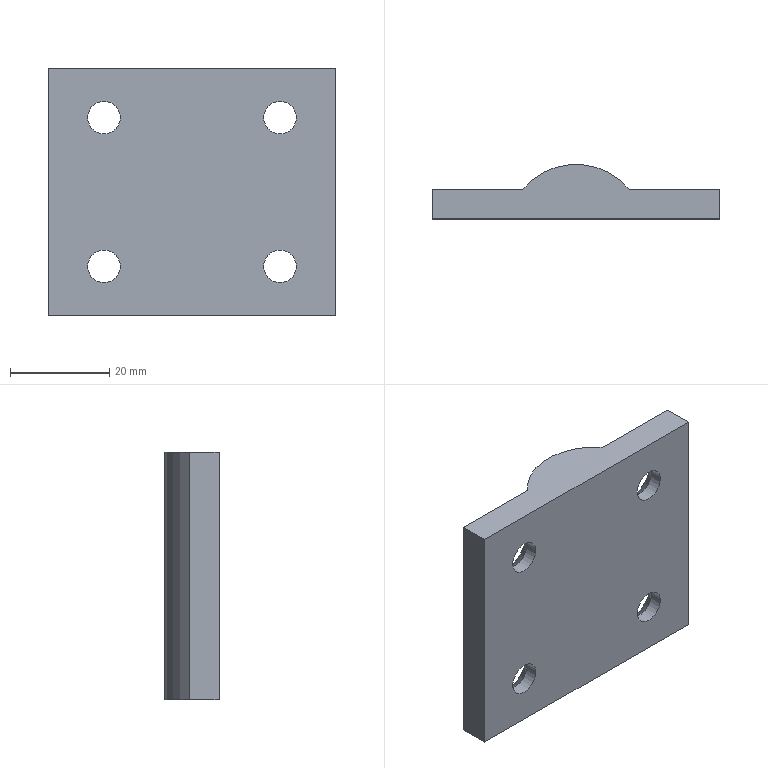Part | SolidWorks | features BaseBody 1 | 1 solid | 24 faces | box 58 x 11 x 50 mm | volume 19652 mm3 | cylinder 9 | cone 8 | plane 7 | commonest cylinder face diameters 6.6 x8 28 x1
STEP:
#1=CARTESIAN_POINT('',(43.45,0.,10.));
#2=VERTEX_POINT('',#1);
#3=CARTESIAN_POINT('',(50.05,0.,10.));
#4=VERTEX_POINT('',#3);
#5=CARTESIAN_POINT('',(46.75,0.,10.));
#6=DIRECTION('',(0.,-1.,0.));
#7=DIRECTION('',(-1.,0.,0.));
#8=AXIS2_PLACEMENT_3D('',#5,#6,#7);
#9=CIRCLE('',#8,3.3);
#10=EDGE_CURVE('',#2,#4,#9,.T.);
#11=ORIENTED_EDGE('',*,*,#10,.T.);
#12=CARTESIAN_POINT('',(50.05,2.58,10.));
#13=VERTEX_POINT('',#12);
#14=CARTESIAN_POINT('',(50.05,6.,10.));
#15=DIRECTION('',(0.,1.,0.));
#16=VECTOR('',#15,1000.);
#17=LINE('',#14,#16);
#18=EDGE_CURVE('',#4,#13,#17,.T.);
#19=ORIENTED_EDGE('',*,*,#18,.T.);
#20=CARTESIAN_POINT('',(43.45,2.58,10.));
#21=VERTEX_POINT('',#20);
#22=CARTESIAN_POINT('',(46.75,2.58,10.));
#23=DIRECTION('',(0.,-1.,0.));
#24=DIRECTION('',(-1.,0.,0.));
#25=AXIS2_PLACEMENT_3D('',#22,#23,#24);
#26=CIRCLE('',#25,3.3);
#27=EDGE_CURVE('',#21,#13,#26,.T.);
#28=ORIENTED_EDGE('',*,*,#27,.F.);
#29=CARTESIAN_POINT('',(43.45,6.,10.));
#30=DIRECTION('',(0.,1.,0.));
#31=VECTOR('',#30,1000.);
#32=LINE('',#29,#31);
#33=EDGE_CURVE('',#2,#21,#32,.T.);
#34=ORIENTED_EDGE('',*,*,#33,.F.);
#35=EDGE_LOOP('',(#11,#19,#28,#34));
#36=FACE_OUTER_BOUND('',#35,.T.);
#37=CARTESIAN_POINT('',(46.75,6.,10.));
#38=DIRECTION('',(0.,1.,0.));
#39=DIRECTION('',(-1.,0.,0.));
#40=AXIS2_PLACEMENT_3D('',#37,#38,#39);
#41=CYLINDRICAL_SURFACE('',#40,3.3);
#42=ADVANCED_FACE('',(#36),#41,.F.);
#43=CARTESIAN_POINT('',(43.45,0.,40.));
#44=VERTEX_POINT('',#43);
#45=CARTESIAN_POINT('',(50.05,0.,40.));
#46=VERTEX_POINT('',#45);
#47=CARTESIAN_POINT('',(46.75,0.,40.));
#48=DIRECTION('',(0.,-1.,0.));
#49=DIRECTION('',(-1.,0.,0.));
#50=AXIS2_PLACEMENT_3D('',#47,#48,#49);
#51=CIRCLE('',#50,3.3);
#52=EDGE_CURVE('',#44,#46,#51,.T.);
#53=ORIENTED_EDGE('',*,*,#52,.T.);
#54=CARTESIAN_POINT('',(50.05,2.58,40.));
#55=VERTEX_POINT('',#54);
#56=CARTESIAN_POINT('',(50.05,6.,40.));
#57=DIRECTION('',(0.,1.,0.));
#58=VECTOR('',#57,1000.);
#59=LINE('',#56,#58);
#60=EDGE_CURVE('',#46,#55,#59,.T.);
#61=ORIENTED_EDGE('',*,*,#60,.T.);
#62=CARTESIAN_POINT('',(43.45,2.58,40.));
#63=VERTEX_POINT('',#62);
#64=CARTESIAN_POINT('',(46.75,2.58,40.));
#65=DIRECTION('',(0.,-1.,0.));
#66=DIRECTION('',(-1.,0.,0.));
#67=AXIS2_PLACEMENT_3D('',#64,#65,#66);
#68=CIRCLE('',#67,3.3);
#69=EDGE_CURVE('',#63,#55,#68,.T.);
#70=ORIENTED_EDGE('',*,*,#69,.F.);
#71=CARTESIAN_POINT('',(43.45,6.,40.));
#72=DIRECTION('',(0.,1.,0.));
#73=VECTOR('',#72,1000.);
#74=LINE('',#71,#73);
#75=EDGE_CURVE('',#44,#63,#74,.T.);
#76=ORIENTED_EDGE('',*,*,#75,.F.);
#77=EDGE_LOOP('',(#53,#61,#70,#76));
#78=FACE_OUTER_BOUND('',#77,.T.);
#79=CARTESIAN_POINT('',(46.75,6.,40.));
#80=DIRECTION('',(0.,1.,0.));
#81=DIRECTION('',(-1.,0.,0.));
#82=AXIS2_PLACEMENT_3D('',#79,#80,#81);
#83=CYLINDRICAL_SURFACE('',#82,3.3);
#84=ADVANCED_FACE('',(#78),#83,.F.);
#85=CARTESIAN_POINT('',(7.95,0.,40.));
#86=VERTEX_POINT('',#85);
#87=CARTESIAN_POINT('',(14.55,0.,40.));
#88=VERTEX_POINT('',#87);
#89=CARTESIAN_POINT('',(11.25,0.,40.));
#90=DIRECTION('',(0.,-1.,0.));
#91=DIRECTION('',(-1.,0.,0.));
#92=AXIS2_PLACEMENT_3D('',#89,#90,#91);
#93=CIRCLE('',#92,3.3);
#94=EDGE_CURVE('',#86,#88,#93,.T.);
#95=ORIENTED_EDGE('',*,*,#94,.T.);
#96=CARTESIAN_POINT('',(14.55,2.58,40.));
#97=VERTEX_POINT('',#96);
#98=CARTESIAN_POINT('',(14.55,6.,40.));
#99=DIRECTION('',(0.,1.,0.));
#100=VECTOR('',#99,1000.);
#101=LINE('',#98,#100);
#102=EDGE_CURVE('',#88,#97,#101,.T.);
#103=ORIENTED_EDGE('',*,*,#102,.T.);
#104=CARTESIAN_POINT('',(7.95,2.58,40.));
#105=VERTEX_POINT('',#104);
#106=CARTESIAN_POINT('',(11.25,2.58,40.));
#107=DIRECTION('',(0.,-1.,0.));
#108=DIRECTION('',(-1.,0.,0.));
#109=AXIS2_PLACEMENT_3D('',#106,#107,#108);
#110=CIRCLE('',#109,3.3);
#111=EDGE_CURVE('',#105,#97,#110,.T.);
#112=ORIENTED_EDGE('',*,*,#111,.F.);
#113=CARTESIAN_POINT('',(7.95,6.,40.));
#114=DIRECTION('',(0.,1.,0.));
#115=VECTOR('',#114,1000.);
#116=LINE('',#113,#115);
#117=EDGE_CURVE('',#86,#105,#116,.T.);
#118=ORIENTED_EDGE('',*,*,#117,.F.);
#119=EDGE_LOOP('',(#95,#103,#112,#118));
#120=FACE_OUTER_BOUND('',#119,.T.);
#121=CARTESIAN_POINT('',(11.25,6.,40.));
#122=DIRECTION('',(0.,1.,0.));
#123=DIRECTION('',(-1.,0.,0.));
#124=AXIS2_PLACEMENT_3D('',#121,#122,#123);
#125=CYLINDRICAL_SURFACE('',#124,3.3);
#126=ADVANCED_FACE('',(#120),#125,.F.);
#127=CARTESIAN_POINT('',(7.95,0.,10.));
#128=VERTEX_POINT('',#127);
#129=CARTESIAN_POINT('',(14.55,0.,10.));
#130=VERTEX_POINT('',#129);
#131=CARTESIAN_POINT('',(11.25,0.,10.));
#132=DIRECTION('',(0.,-1.,0.));
#133=DIRECTION('',(-1.,0.,0.));
#134=AXIS2_PLACEMENT_3D('',#131,#132,#133);
#135=CIRCLE('',#134,3.3);
#136=EDGE_CURVE('',#128,#130,#135,.T.);
#137=ORIENTED_EDGE('',*,*,#136,.T.);
#138=CARTESIAN_POINT('',(14.55,2.58,10.));
#139=VERTEX_POINT('',#138);
#140=CARTESIAN_POINT('',(14.55,6.,10.));
#141=DIRECTION('',(0.,1.,0.));
#142=VECTOR('',#141,1000.);
#143=LINE('',#140,#142);
#144=EDGE_CURVE('',#130,#139,#143,.T.);
#145=ORIENTED_EDGE('',*,*,#144,.T.);
#146=CARTESIAN_POINT('',(7.95,2.58,10.));
#147=VERTEX_POINT('',#146);
#148=CARTESIAN_POINT('',(11.25,2.58,10.));
#149=DIRECTION('',(0.,-1.,0.));
#150=DIRECTION('',(-1.,0.,0.));
#151=AXIS2_PLACEMENT_3D('',#148,#149,#150);
#152=CIRCLE('',#151,3.3);
#153=EDGE_CURVE('',#147,#139,#152,.T.);
#154=ORIENTED_EDGE('',*,*,#153,.F.);
#155=CARTESIAN_POINT('',(7.95,6.,10.));
#156=DIRECTION('',(0.,1.,0.));
#157=VECTOR('',#156,1000.);
#158=LINE('',#155,#157);
#159=EDGE_CURVE('',#128,#147,#158,.T.);
#160=ORIENTED_EDGE('',*,*,#159,.F.);
#161=EDGE_LOOP('',(#137,#145,#154,#160));
#162=FACE_OUTER_BOUND('',#161,.T.);
#163=CARTESIAN_POINT('',(11.25,6.,10.));
#164=DIRECTION('',(0.,1.,0.));
#165=DIRECTION('',(-1.,0.,0.));
#166=AXIS2_PLACEMENT_3D('',#163,#164,#165);
#167=CYLINDRICAL_SURFACE('',#166,3.3);
#168=ADVANCED_FACE('',(#162),#167,.F.);
#169=ORIENTED_EDGE('',*,*,#27,.T.);
#170=CARTESIAN_POINT('',(53.47,6.,10.));
#171=VERTEX_POINT('',#170);
#172=CARTESIAN_POINT('',(53.47,6.,10.));
#173=DIRECTION('',(0.7071,0.7071,0.));
#174=VECTOR('',#173,1000.);
#175=LINE('',#172,#174);
#176=EDGE_CURVE('',#13,#171,#175,.T.);
#177=ORIENTED_EDGE('',*,*,#176,.T.);
#178=CARTESIAN_POINT('',(40.03,6.,10.));
#179=VERTEX_POINT('',#178);
#180=CARTESIAN_POINT('',(46.75,6.,10.));
#181=DIRECTION('',(0.,1.,0.));
#182=DIRECTION('',(-1.,0.,0.));
#183=AXIS2_PLACEMENT_3D('',#180,#181,#182);
#184=CIRCLE('',#183,6.72);
#185=EDGE_CURVE('',#171,#179,#184,.T.);
#186=ORIENTED_EDGE('',*,*,#185,.T.);
#187=CARTESIAN_POINT('',(40.03,6.,10.));
#188=DIRECTION('',(-0.7071,0.7071,0.));
#189=VECTOR('',#188,1000.);
#190=LINE('',#187,#189);
#191=EDGE_CURVE('',#21,#179,#190,.T.);
#192=ORIENTED_EDGE('',*,*,#191,.F.);
#193=EDGE_LOOP('',(#169,#177,#186,#192));
#194=FACE_OUTER_BOUND('',#193,.T.);
#195=CARTESIAN_POINT('',(46.75,6.,10.));
#196=DIRECTION('',(0.,1.,0.));
#197=DIRECTION('',(-1.,0.,0.));
#198=AXIS2_PLACEMENT_3D('',#195,#196,#197);
#199=CONICAL_SURFACE('',#198,6.72,0.7854);
#200=ADVANCED_FACE('',(#194),#199,.F.);
#201=ORIENTED_EDGE('',*,*,#69,.T.);
#202=CARTESIAN_POINT('',(53.47,6.,40.));
#203=VERTEX_POINT('',#202);
#204=CARTESIAN_POINT('',(53.47,6.,40.));
#205=DIRECTION('',(0.7071,0.7071,0.));
#206=VECTOR('',#205,1000.);
#207=LINE('',#204,#206);
#208=EDGE_CURVE('',#55,#203,#207,.T.);
#209=ORIENTED_EDGE('',*,*,#208,.T.);
#210=CARTESIAN_POINT('',(40.03,6.,40.));
#211=VERTEX_POINT('',#210);
#212=CARTESIAN_POINT('',(46.75,6.,40.));
#213=DIRECTION('',(0.,1.,0.));
#214=DIRECTION('',(-1.,0.,0.));
#215=AXIS2_PLACEMENT_3D('',#212,#213,#214);
#216=CIRCLE('',#215,6.72);
#217=EDGE_CURVE('',#203,#211,#216,.T.);
#218=ORIENTED_EDGE('',*,*,#217,.T.);
#219=CARTESIAN_POINT('',(40.03,6.,40.));
#220=DIRECTION('',(-0.7071,0.7071,0.));
#221=VECTOR('',#220,1000.);
#222=LINE('',#219,#221);
#223=EDGE_CURVE('',#63,#211,#222,.T.);
#224=ORIENTED_EDGE('',*,*,#223,.F.);
#225=EDGE_LOOP('',(#201,#209,#218,#224));
#226=FACE_OUTER_BOUND('',#225,.T.);
#227=CARTESIAN_POINT('',(46.75,6.,40.));
#228=DIRECTION('',(0.,1.,0.));
#229=DIRECTION('',(-1.,0.,0.));
#230=AXIS2_PLACEMENT_3D('',#227,#228,#229);
#231=CONICAL_SURFACE('',#230,6.72,0.7854);
#232=ADVANCED_FACE('',(#226),#231,.F.);
#233=ORIENTED_EDGE('',*,*,#111,.T.);
#234=CARTESIAN_POINT('',(17.97,6.,40.));
#235=VERTEX_POINT('',#234);
#236=CARTESIAN_POINT('',(17.97,6.,40.));
#237=DIRECTION('',(0.7071,0.7071,0.));
#238=VECTOR('',#237,1000.);
#239=LINE('',#236,#238);
#240=EDGE_CURVE('',#97,#235,#239,.T.);
#241=ORIENTED_EDGE('',*,*,#240,.T.);
#242=CARTESIAN_POINT('',(4.53,6.,40.));
#243=VERTEX_POINT('',#242);
#244=CARTESIAN_POINT('',(11.25,6.,40.));
#245=DIRECTION('',(0.,1.,0.));
#246=DIRECTION('',(-1.,0.,0.));
#247=AXIS2_PLACEMENT_3D('',#244,#245,#246);
#248=CIRCLE('',#247,6.72);
#249=EDGE_CURVE('',#235,#243,#248,.T.);
#250=ORIENTED_EDGE('',*,*,#249,.T.);
#251=CARTESIAN_POINT('',(4.53,6.,40.));
#252=DIRECTION('',(-0.7071,0.7071,0.));
#253=VECTOR('',#252,1000.);
#254=LINE('',#251,#253);
#255=EDGE_CURVE('',#105,#243,#254,.T.);
#256=ORIENTED_EDGE('',*,*,#255,.F.);
#257=EDGE_LOOP('',(#233,#241,#250,#256));
#258=FACE_OUTER_BOUND('',#257,.T.);
#259=CARTESIAN_POINT('',(11.25,6.,40.));
#260=DIRECTION('',(0.,1.,0.));
#261=DIRECTION('',(-1.,0.,0.));
#262=AXIS2_PLACEMENT_3D('',#259,#260,#261);
#263=CONICAL_SURFACE('',#262,6.72,0.7854);
#264=ADVANCED_FACE('',(#258),#263,.F.);
#265=ORIENTED_EDGE('',*,*,#153,.T.);
#266=CARTESIAN_POINT('',(17.97,6.,10.));
#267=VERTEX_POINT('',#266);
#268=CARTESIAN_POINT('',(17.97,6.,10.));
#269=DIRECTION('',(0.7071,0.7071,0.));
#270=VECTOR('',#269,1000.);
#271=LINE('',#268,#270);
#272=EDGE_CURVE('',#139,#267,#271,.T.);
#273=ORIENTED_EDGE('',*,*,#272,.T.);
#274=CARTESIAN_POINT('',(4.53,6.,10.));
#275=VERTEX_POINT('',#274);
#276=CARTESIAN_POINT('',(11.25,6.,10.));
#277=DIRECTION('',(0.,1.,0.));
#278=DIRECTION('',(-1.,0.,0.));
#279=AXIS2_PLACEMENT_3D('',#276,#277,#278);
#280=CIRCLE('',#279,6.72);
#281=EDGE_CURVE('',#267,#275,#280,.T.);
#282=ORIENTED_EDGE('',*,*,#281,.T.);
#283=CARTESIAN_POINT('',(4.53,6.,10.));
#284=DIRECTION('',(-0.7071,0.7071,0.));
#285=VECTOR('',#284,1000.);
#286=LINE('',#283,#285);
#287=EDGE_CURVE('',#147,#275,#286,.T.);
#288=ORIENTED_EDGE('',*,*,#287,.F.);
#289=EDGE_LOOP('',(#265,#273,#282,#288));
#290=FACE_OUTER_BOUND('',#289,.T.);
#291=CARTESIAN_POINT('',(11.25,6.,10.));
#292=DIRECTION('',(0.,1.,0.));
#293=DIRECTION('',(-1.,0.,0.));
#294=AXIS2_PLACEMENT_3D('',#291,#292,#293);
#295=CONICAL_SURFACE('',#294,6.72,0.7854);
#296=ADVANCED_FACE('',(#290),#295,.F.);
#297=CARTESIAN_POINT('',(58.,0.,50.));
#298=VERTEX_POINT('',#297);
#299=CARTESIAN_POINT('',(58.,0.,0.));
#300=VERTEX_POINT('',#299);
#301=CARTESIAN_POINT('',(58.,0.,50.));
#302=DIRECTION('',(0.,0.,-1.));
#303=VECTOR('',#302,1000.);
#304=LINE('',#301,#303);
#305=EDGE_CURVE('',#298,#300,#304,.T.);
#306=ORIENTED_EDGE('',*,*,#305,.F.);
#307=CARTESIAN_POINT('',(0.,0.,50.));
#308=VERTEX_POINT('',#307);
#309=CARTESIAN_POINT('',(0.,0.,50.));
#310=DIRECTION('',(1.,0.,0.));
#311=VECTOR('',#310,1000.);
#312=LINE('',#309,#311);
#313=EDGE_CURVE('',#308,#298,#312,.T.);
#314=ORIENTED_EDGE('',*,*,#313,.F.);
#315=CARTESIAN_POINT('',(0.,0.,0.));
#316=VERTEX_POINT('',#315);
#317=CARTESIAN_POINT('',(0.,0.,50.));
#318=DIRECTION('',(0.,0.,1.));
#319=VECTOR('',#318,1000.);
#320=LINE('',#317,#319);
#321=EDGE_CURVE('',#316,#308,#320,.T.);
#322=ORIENTED_EDGE('',*,*,#321,.F.);
#323=CARTESIAN_POINT('',(0.,0.,0.));
#324=DIRECTION('',(-1.,0.,0.));
#325=VECTOR('',#324,1000.);
#326=LINE('',#323,#325);
#327=EDGE_CURVE('',#300,#316,#326,.T.);
#328=ORIENTED_EDGE('',*,*,#327,.F.);
#329=EDGE_LOOP('',(#306,#314,#322,#328));
#330=FACE_OUTER_BOUND('',#329,.T.);
#331=ORIENTED_EDGE('',*,*,#10,.F.);
#332=CARTESIAN_POINT('',(46.75,0.,10.));
#333=DIRECTION('',(0.,-1.,0.));
#334=DIRECTION('',(-1.,0.,0.));
#335=AXIS2_PLACEMENT_3D('',#332,#333,#334);
#336=CIRCLE('',#335,3.3);
#337=EDGE_CURVE('',#4,#2,#336,.T.);
#338=ORIENTED_EDGE('',*,*,#337,.F.);
#339=EDGE_LOOP('',(#331,#338));
#340=FACE_BOUND('',#339,.T.);
#341=ORIENTED_EDGE('',*,*,#52,.F.);
#342=CARTESIAN_POINT('',(46.75,0.,40.));
#343=DIRECTION('',(0.,-1.,0.));
#344=DIRECTION('',(-1.,0.,0.));
#345=AXIS2_PLACEMENT_3D('',#342,#343,#344);
#346=CIRCLE('',#345,3.3);
#347=EDGE_CURVE('',#46,#44,#346,.T.);
#348=ORIENTED_EDGE('',*,*,#347,.F.);
#349=EDGE_LOOP('',(#341,#348));
#350=FACE_BOUND('',#349,.T.);
#351=ORIENTED_EDGE('',*,*,#94,.F.);
#352=CARTESIAN_POINT('',(11.25,0.,40.));
#353=DIRECTION('',(0.,-1.,0.));
#354=DIRECTION('',(-1.,0.,0.));
#355=AXIS2_PLACEMENT_3D('',#352,#353,#354);
#356=CIRCLE('',#355,3.3);
#357=EDGE_CURVE('',#88,#86,#356,.T.);
#358=ORIENTED_EDGE('',*,*,#357,.F.);
#359=EDGE_LOOP('',(#351,#358));
#360=FACE_BOUND('',#359,.T.);
#361=ORIENTED_EDGE('',*,*,#136,.F.);
#362=CARTESIAN_POINT('',(11.25,0.,10.));
#363=DIRECTION('',(0.,-1.,0.));
#364=DIRECTION('',(-1.,0.,0.));
#365=AXIS2_PLACEMENT_3D('',#362,#363,#364);
#366=CIRCLE('',#365,3.3);
#367=EDGE_CURVE('',#130,#128,#366,.T.);
#368=ORIENTED_EDGE('',*,*,#367,.F.);
#369=EDGE_LOOP('',(#361,#368));
#370=FACE_BOUND('',#369,.T.);
#371=CARTESIAN_POINT('',(0.,0.,50.));
#372=DIRECTION('',(0.,1.,0.));
#373=DIRECTION('',(-1.,0.,0.));
#374=AXIS2_PLACEMENT_3D('',#371,#372,#373);
#375=PLANE('',#374);
#376=ADVANCED_FACE('',(#330,#340,#350,#360,#370),#375,.F.);
#377=CARTESIAN_POINT('',(18.276,6.,0.));
#378=VERTEX_POINT('',#377);
#379=CARTESIAN_POINT('',(0.,6.,0.));
#380=VERTEX_POINT('',#379);
#381=CARTESIAN_POINT('',(29.,6.,0.));
#382=DIRECTION('',(-1.,0.,0.));
#383=VECTOR('',#382,1000.);
#384=LINE('',#381,#383);
#385=EDGE_CURVE('',#378,#380,#384,.T.);
#386=ORIENTED_EDGE('',*,*,#385,.F.);
#387=CARTESIAN_POINT('',(39.724,6.,0.));
#388=VERTEX_POINT('',#387);
#389=CARTESIAN_POINT('',(29.,-3.,0.));
#390=DIRECTION('',(0.,0.,1.));
#391=DIRECTION('',(-1.,0.,0.));
#392=AXIS2_PLACEMENT_3D('',#389,#390,#391);
#393=CIRCLE('',#392,14.);
#394=EDGE_CURVE('',#388,#378,#393,.T.);
#395=ORIENTED_EDGE('',*,*,#394,.F.);
#396=CARTESIAN_POINT('',(58.,6.,0.));
#397=VERTEX_POINT('',#396);
#398=CARTESIAN_POINT('',(29.,6.,0.));
#399=DIRECTION('',(-1.,0.,0.));
#400=VECTOR('',#399,1000.);
#401=LINE('',#398,#400);
#402=EDGE_CURVE('',#397,#388,#401,.T.);
#403=ORIENTED_EDGE('',*,*,#402,.F.);
#404=CARTESIAN_POINT('',(58.,-3.,0.));
#405=DIRECTION('',(0.,1.,0.));
#406=VECTOR('',#405,1000.);
#407=LINE('',#404,#406);
#408=EDGE_CURVE('',#300,#397,#407,.T.);
#409=ORIENTED_EDGE('',*,*,#408,.F.);
#410=ORIENTED_EDGE('',*,*,#327,.T.);
#411=CARTESIAN_POINT('',(0.,-3.,0.));
#412=DIRECTION('',(0.,-1.,0.));
#413=VECTOR('',#412,1000.);
#414=LINE('',#411,#413);
#415=EDGE_CURVE('',#380,#316,#414,.T.);
#416=ORIENTED_EDGE('',*,*,#415,.F.);
#417=EDGE_LOOP('',(#386,#395,#403,#409,#410,#416));
#418=FACE_OUTER_BOUND('',#417,.T.);
#419=CARTESIAN_POINT('',(29.,-3.,0.));
#420=DIRECTION('',(0.,0.,1.));
#421=DIRECTION('',(1.,0.,0.));
#422=AXIS2_PLACEMENT_3D('',#419,#420,#421);
#423=PLANE('',#422);
#424=ADVANCED_FACE('',(#418),#423,.F.);
#425=CARTESIAN_POINT('',(58.,6.,50.));
#426=VERTEX_POINT('',#425);
#427=CARTESIAN_POINT('',(58.,6.,50.));
#428=DIRECTION('',(0.,0.,-1.));
#429=VECTOR('',#428,1000.);
#430=LINE('',#427,#429);
#431=EDGE_CURVE('',#426,#397,#430,.T.);
#432=ORIENTED_EDGE('',*,*,#431,.F.);
#433=CARTESIAN_POINT('',(58.,0.,50.));
#434=DIRECTION('',(0.,1.,0.));
#435=VECTOR('',#434,1000.);
#436=LINE('',#433,#435);
#437=EDGE_CURVE('',#298,#426,#436,.T.);
#438=ORIENTED_EDGE('',*,*,#437,.F.);
#439=ORIENTED_EDGE('',*,*,#305,.T.);
#440=ORIENTED_EDGE('',*,*,#408,.T.);
#441=EDGE_LOOP('',(#432,#438,#439,#440));
#442=FACE_OUTER_BOUND('',#441,.T.);
#443=CARTESIAN_POINT('',(58.,0.,50.));
#444=DIRECTION('',(-1.,0.,0.));
#445=DIRECTION('',(0.,0.,1.));
#446=AXIS2_PLACEMENT_3D('',#443,#444,#445);
#447=PLANE('',#446);
#448=ADVANCED_FACE('',(#442),#447,.F.);
#449=CARTESIAN_POINT('',(39.724,6.,50.));
#450=VERTEX_POINT('',#449);
#451=CARTESIAN_POINT('',(18.276,6.,50.));
#452=VERTEX_POINT('',#451);
#453=CARTESIAN_POINT('',(29.,-3.,50.));
#454=DIRECTION('',(0.,0.,1.));
#455=DIRECTION('',(-1.,0.,0.));
#456=AXIS2_PLACEMENT_3D('',#453,#454,#455);
#457=CIRCLE('',#456,14.);
#458=EDGE_CURVE('',#450,#452,#457,.T.);
#459=ORIENTED_EDGE('',*,*,#458,.T.);
#460=CARTESIAN_POINT('',(0.,6.,50.));
#461=VERTEX_POINT('',#460);
#462=CARTESIAN_POINT('',(29.,6.,50.));
#463=DIRECTION('',(-1.,0.,0.));
#464=VECTOR('',#463,1000.);
#465=LINE('',#462,#464);
#466=EDGE_CURVE('',#452,#461,#465,.T.);
#467=ORIENTED_EDGE('',*,*,#466,.T.);
#468=CARTESIAN_POINT('',(0.,-3.,50.));
#469=DIRECTION('',(0.,-1.,0.));
#470=VECTOR('',#469,1000.);
#471=LINE('',#468,#470);
#472=EDGE_CURVE('',#461,#308,#471,.T.);
#473=ORIENTED_EDGE('',*,*,#472,.T.);
#474=ORIENTED_EDGE('',*,*,#313,.T.);
#475=ORIENTED_EDGE('',*,*,#437,.T.);
#476=CARTESIAN_POINT('',(29.,6.,50.));
#477=DIRECTION('',(-1.,0.,0.));
#478=VECTOR('',#477,1000.);
#479=LINE('',#476,#478);
#480=EDGE_CURVE('',#426,#450,#479,.T.);
#481=ORIENTED_EDGE('',*,*,#480,.T.);
#482=EDGE_LOOP('',(#459,#467,#473,#474,#475,#481));
#483=FACE_OUTER_BOUND('',#482,.T.);
#484=CARTESIAN_POINT('',(29.,-3.,50.));
#485=DIRECTION('',(0.,0.,1.));
#486=DIRECTION('',(1.,0.,0.));
#487=AXIS2_PLACEMENT_3D('',#484,#485,#486);
#488=PLANE('',#487);
#489=ADVANCED_FACE('',(#483),#488,.T.);
#490=ORIENTED_EDGE('',*,*,#321,.T.);
#491=ORIENTED_EDGE('',*,*,#472,.F.);
#492=CARTESIAN_POINT('',(0.,6.,50.));
#493=DIRECTION('',(0.,0.,1.));
#494=VECTOR('',#493,1000.);
#495=LINE('',#492,#494);
#496=EDGE_CURVE('',#380,#461,#495,.T.);
#497=ORIENTED_EDGE('',*,*,#496,.F.);
#498=ORIENTED_EDGE('',*,*,#415,.T.);
#499=EDGE_LOOP('',(#490,#491,#497,#498));
#500=FACE_OUTER_BOUND('',#499,.T.);
#501=CARTESIAN_POINT('',(0.,6.,50.));
#502=DIRECTION('',(1.,0.,0.));
#503=DIRECTION('',(0.,0.,-1.));
#504=AXIS2_PLACEMENT_3D('',#501,#502,#503);
#505=PLANE('',#504);
#506=ADVANCED_FACE('',(#500),#505,.F.);
#507=ORIENTED_EDGE('',*,*,#18,.F.);
#508=ORIENTED_EDGE('',*,*,#337,.T.);
#509=ORIENTED_EDGE('',*,*,#33,.T.);
#510=CARTESIAN_POINT('',(46.75,2.58,10.));
#511=DIRECTION('',(0.,-1.,0.));
#512=DIRECTION('',(-1.,0.,0.));
#513=AXIS2_PLACEMENT_3D('',#510,#511,#512);
#514=CIRCLE('',#513,3.3);
#515=EDGE_CURVE('',#13,#21,#514,.T.);
#516=ORIENTED_EDGE('',*,*,#515,.F.);
#517=EDGE_LOOP('',(#507,#508,#509,#516));
#518=FACE_OUTER_BOUND('',#517,.T.);
#519=CARTESIAN_POINT('',(46.75,6.,10.));
#520=DIRECTION('',(0.,1.,0.));
#521=DIRECTION('',(-1.,0.,0.));
#522=AXIS2_PLACEMENT_3D('',#519,#520,#521);
#523=CYLINDRICAL_SURFACE('',#522,3.3);
#524=ADVANCED_FACE('',(#518),#523,.F.);
#525=ORIENTED_EDGE('',*,*,#60,.F.);
#526=ORIENTED_EDGE('',*,*,#347,.T.);
#527=ORIENTED_EDGE('',*,*,#75,.T.);
#528=CARTESIAN_POINT('',(46.75,2.58,40.));
#529=DIRECTION('',(0.,-1.,0.));
#530=DIRECTION('',(-1.,0.,0.));
#531=AXIS2_PLACEMENT_3D('',#528,#529,#530);
#532=CIRCLE('',#531,3.3);
#533=EDGE_CURVE('',#55,#63,#532,.T.);
#534=ORIENTED_EDGE('',*,*,#533,.F.);
#535=EDGE_LOOP('',(#525,#526,#527,#534));
#536=FACE_OUTER_BOUND('',#535,.T.);
#537=CARTESIAN_POINT('',(46.75,6.,40.));
#538=DIRECTION('',(0.,1.,0.));
#539=DIRECTION('',(-1.,0.,0.));
#540=AXIS2_PLACEMENT_3D('',#537,#538,#539);
#541=CYLINDRICAL_SURFACE('',#540,3.3);
#542=ADVANCED_FACE('',(#536),#541,.F.);
#543=ORIENTED_EDGE('',*,*,#102,.F.);
#544=ORIENTED_EDGE('',*,*,#357,.T.);
#545=ORIENTED_EDGE('',*,*,#117,.T.);
#546=CARTESIAN_POINT('',(11.25,2.58,40.));
#547=DIRECTION('',(0.,-1.,0.));
#548=DIRECTION('',(-1.,0.,0.));
#549=AXIS2_PLACEMENT_3D('',#546,#547,#548);
#550=CIRCLE('',#549,3.3);
#551=EDGE_CURVE('',#97,#105,#550,.T.);
#552=ORIENTED_EDGE('',*,*,#551,.F.);
#553=EDGE_LOOP('',(#543,#544,#545,#552));
#554=FACE_OUTER_BOUND('',#553,.T.);
#555=CARTESIAN_POINT('',(11.25,6.,40.));
#556=DIRECTION('',(0.,1.,0.));
#557=DIRECTION('',(-1.,0.,0.));
#558=AXIS2_PLACEMENT_3D('',#555,#556,#557);
#559=CYLINDRICAL_SURFACE('',#558,3.3);
#560=ADVANCED_FACE('',(#554),#559,.F.);
#561=ORIENTED_EDGE('',*,*,#144,.F.);
#562=ORIENTED_EDGE('',*,*,#367,.T.);
#563=ORIENTED_EDGE('',*,*,#159,.T.);
#564=CARTESIAN_POINT('',(11.25,2.58,10.));
#565=DIRECTION('',(0.,-1.,0.));
#566=DIRECTION('',(-1.,0.,0.));
#567=AXIS2_PLACEMENT_3D('',#564,#565,#566);
#568=CIRCLE('',#567,3.3);
#569=EDGE_CURVE('',#139,#147,#568,.T.);
#570=ORIENTED_EDGE('',*,*,#569,.F.);
#571=EDGE_LOOP('',(#561,#562,#563,#570));
#572=FACE_OUTER_BOUND('',#571,.T.);
#573=CARTESIAN_POINT('',(11.25,6.,10.));
#574=DIRECTION('',(0.,1.,0.));
#575=DIRECTION('',(-1.,0.,0.));
#576=AXIS2_PLACEMENT_3D('',#573,#574,#575);
#577=CYLINDRICAL_SURFACE('',#576,3.3);
#578=ADVANCED_FACE('',(#572),#577,.F.);
#579=ORIENTED_EDGE('',*,*,#496,.T.);
#580=ORIENTED_EDGE('',*,*,#466,.F.);
#581=CARTESIAN_POINT('',(18.276,6.,50.));
#582=DIRECTION('',(0.,0.,1.));
#583=VECTOR('',#582,1000.);
#584=LINE('',#581,#583);
#585=EDGE_CURVE('',#378,#452,#584,.T.);
#586=ORIENTED_EDGE('',*,*,#585,.F.);
#587=ORIENTED_EDGE('',*,*,#385,.T.);
#588=EDGE_LOOP('',(#579,#580,#586,#587));
#589=FACE_OUTER_BOUND('',#588,.T.);
#590=CARTESIAN_POINT('',(11.25,6.,40.));
#591=DIRECTION('',(0.,1.,0.));
#592=DIRECTION('',(-1.,0.,0.));
#593=AXIS2_PLACEMENT_3D('',#590,#591,#592);
#594=CIRCLE('',#593,6.72);
#595=EDGE_CURVE('',#243,#235,#594,.T.);
#596=ORIENTED_EDGE('',*,*,#595,.F.);
#597=ORIENTED_EDGE('',*,*,#249,.F.);
#598=EDGE_LOOP('',(#596,#597));
#599=FACE_BOUND('',#598,.T.);
#600=CARTESIAN_POINT('',(11.25,6.,10.));
#601=DIRECTION('',(0.,1.,0.));
#602=DIRECTION('',(-1.,0.,0.));
#603=AXIS2_PLACEMENT_3D('',#600,#601,#602);
#604=CIRCLE('',#603,6.72);
#605=EDGE_CURVE('',#275,#267,#604,.T.);
#606=ORIENTED_EDGE('',*,*,#605,.F.);
#607=ORIENTED_EDGE('',*,*,#281,.F.);
#608=EDGE_LOOP('',(#606,#607));
#609=FACE_BOUND('',#608,.T.);
#610=CARTESIAN_POINT('',(18.276,6.,50.));
#611=DIRECTION('',(0.,-1.,0.));
#612=DIRECTION('',(1.,0.,0.));
#613=AXIS2_PLACEMENT_3D('',#610,#611,#612);
#614=PLANE('',#613);
#615=ADVANCED_FACE('',(#589,#599,#609),#614,.F.);
#616=ORIENTED_EDGE('',*,*,#458,.F.);
#617=CARTESIAN_POINT('',(39.724,6.,50.));
#618=DIRECTION('',(0.,0.,-1.));
#619=VECTOR('',#618,1000.);
#620=LINE('',#617,#619);
#621=EDGE_CURVE('',#450,#388,#620,.T.);
#622=ORIENTED_EDGE('',*,*,#621,.T.);
#623=ORIENTED_EDGE('',*,*,#394,.T.);
#624=ORIENTED_EDGE('',*,*,#585,.T.);
#625=EDGE_LOOP('',(#616,#622,#623,#624));
#626=FACE_OUTER_BOUND('',#625,.T.);
#627=CARTESIAN_POINT('',(29.,-3.,50.));
#628=DIRECTION('',(0.,0.,-1.));
#629=DIRECTION('',(-1.,0.,0.));
#630=AXIS2_PLACEMENT_3D('',#627,#628,#629);
#631=CYLINDRICAL_SURFACE('',#630,14.);
#632=ADVANCED_FACE('',(#626),#631,.T.);
#633=ORIENTED_EDGE('',*,*,#621,.F.);
#634=ORIENTED_EDGE('',*,*,#480,.F.);
#635=ORIENTED_EDGE('',*,*,#431,.T.);
#636=ORIENTED_EDGE('',*,*,#402,.T.);
#637=EDGE_LOOP('',(#633,#634,#635,#636));
#638=FACE_OUTER_BOUND('',#637,.T.);
#639=CARTESIAN_POINT('',(46.75,6.,10.));
#640=DIRECTION('',(0.,1.,0.));
#641=DIRECTION('',(-1.,0.,0.));
#642=AXIS2_PLACEMENT_3D('',#639,#640,#641);
#643=CIRCLE('',#642,6.72);
#644=EDGE_CURVE('',#179,#171,#643,.T.);
#645=ORIENTED_EDGE('',*,*,#644,.F.);
#646=ORIENTED_EDGE('',*,*,#185,.F.);
#647=EDGE_LOOP('',(#645,#646));
#648=FACE_BOUND('',#647,.T.);
#649=CARTESIAN_POINT('',(46.75,6.,40.));
#650=DIRECTION('',(0.,1.,0.));
#651=DIRECTION('',(-1.,0.,0.));
#652=AXIS2_PLACEMENT_3D('',#649,#650,#651);
#653=CIRCLE('',#652,6.72);
#654=EDGE_CURVE('',#211,#203,#653,.T.);
#655=ORIENTED_EDGE('',*,*,#654,.F.);
#656=ORIENTED_EDGE('',*,*,#217,.F.);
#657=EDGE_LOOP('',(#655,#656));
#658=FACE_BOUND('',#657,.T.);
#659=CARTESIAN_POINT('',(58.,6.,50.));
#660=DIRECTION('',(0.,-1.,0.));
#661=DIRECTION('',(1.,0.,0.));
#662=AXIS2_PLACEMENT_3D('',#659,#660,#661);
#663=PLANE('',#662);
#664=ADVANCED_FACE('',(#638,#648,#658),#663,.F.);
#665=ORIENTED_EDGE('',*,*,#176,.F.);
#666=ORIENTED_EDGE('',*,*,#515,.T.);
#667=ORIENTED_EDGE('',*,*,#191,.T.);
#668=ORIENTED_EDGE('',*,*,#644,.T.);
#669=EDGE_LOOP('',(#665,#666,#667,#668));
#670=FACE_OUTER_BOUND('',#669,.T.);
#671=CARTESIAN_POINT('',(46.75,6.,10.));
#672=DIRECTION('',(0.,1.,0.));
#673=DIRECTION('',(-1.,0.,0.));
#674=AXIS2_PLACEMENT_3D('',#671,#672,#673);
#675=CONICAL_SURFACE('',#674,6.72,0.7854);
#676=ADVANCED_FACE('',(#670),#675,.F.);
#677=ORIENTED_EDGE('',*,*,#208,.F.);
#678=ORIENTED_EDGE('',*,*,#533,.T.);
#679=ORIENTED_EDGE('',*,*,#223,.T.);
#680=ORIENTED_EDGE('',*,*,#654,.T.);
#681=EDGE_LOOP('',(#677,#678,#679,#680));
#682=FACE_OUTER_BOUND('',#681,.T.);
#683=CARTESIAN_POINT('',(46.75,6.,40.));
#684=DIRECTION('',(0.,1.,0.));
#685=DIRECTION('',(-1.,0.,0.));
#686=AXIS2_PLACEMENT_3D('',#683,#684,#685);
#687=CONICAL_SURFACE('',#686,6.72,0.7854);
#688=ADVANCED_FACE('',(#682),#687,.F.);
#689=ORIENTED_EDGE('',*,*,#240,.F.);
#690=ORIENTED_EDGE('',*,*,#551,.T.);
#691=ORIENTED_EDGE('',*,*,#255,.T.);
#692=ORIENTED_EDGE('',*,*,#595,.T.);
#693=EDGE_LOOP('',(#689,#690,#691,#692));
#694=FACE_OUTER_BOUND('',#693,.T.);
#695=CARTESIAN_POINT('',(11.25,6.,40.));
#696=DIRECTION('',(0.,1.,0.));
#697=DIRECTION('',(-1.,0.,0.));
#698=AXIS2_PLACEMENT_3D('',#695,#696,#697);
#699=CONICAL_SURFACE('',#698,6.72,0.7854);
#700=ADVANCED_FACE('',(#694),#699,.F.);
#701=ORIENTED_EDGE('',*,*,#272,.F.);
#702=ORIENTED_EDGE('',*,*,#569,.T.);
#703=ORIENTED_EDGE('',*,*,#287,.T.);
#704=ORIENTED_EDGE('',*,*,#605,.T.);
#705=EDGE_LOOP('',(#701,#702,#703,#704));
#706=FACE_OUTER_BOUND('',#705,.T.);
#707=CARTESIAN_POINT('',(11.25,6.,10.));
#708=DIRECTION('',(0.,1.,0.));
#709=DIRECTION('',(-1.,0.,0.));
#710=AXIS2_PLACEMENT_3D('',#707,#708,#709);
#711=CONICAL_SURFACE('',#710,6.72,0.7854);
#712=ADVANCED_FACE('',(#706),#711,.F.);
#713=CLOSED_SHELL('',(#42,#84,#126,#168,#200,#232,#264,#296,#376,#424,#448,#489,#506,#524,#542,#560,#578,#615,#632,#664,#676,#688,#700,#712));
#714=MANIFOLD_SOLID_BREP('',#713);
#715=CARTESIAN_POINT('',(0.,0.,0.));
#716=DIRECTION('',(0.,0.,1.));
#717=DIRECTION('',(1.,0.,0.));
#718=AXIS2_PLACEMENT_3D('',#715,#716,#717);
#719=(LENGTH_UNIT()NAMED_UNIT(*)SI_UNIT(.MILLI.,.METRE.));
#720=UNCERTAINTY_MEASURE_WITH_UNIT(LENGTH_MEASURE(0.00001),#719,'','');
#721=(NAMED_UNIT(*)PLANE_ANGLE_UNIT()SI_UNIT($,.RADIAN.));
#722=(NAMED_UNIT(*)SI_UNIT($,.STERADIAN.)SOLID_ANGLE_UNIT());
#723=(GEOMETRIC_REPRESENTATION_CONTEXT(3)GLOBAL_UNCERTAINTY_ASSIGNED_CONTEXT((#720))GLOBAL_UNIT_ASSIGNED_CONTEXT((#719,#721,#722))REPRESENTATION_CONTEXT('',''));
#724=ADVANCED_BREP_SHAPE_REPRESENTATION('',(#714,#718),#723);